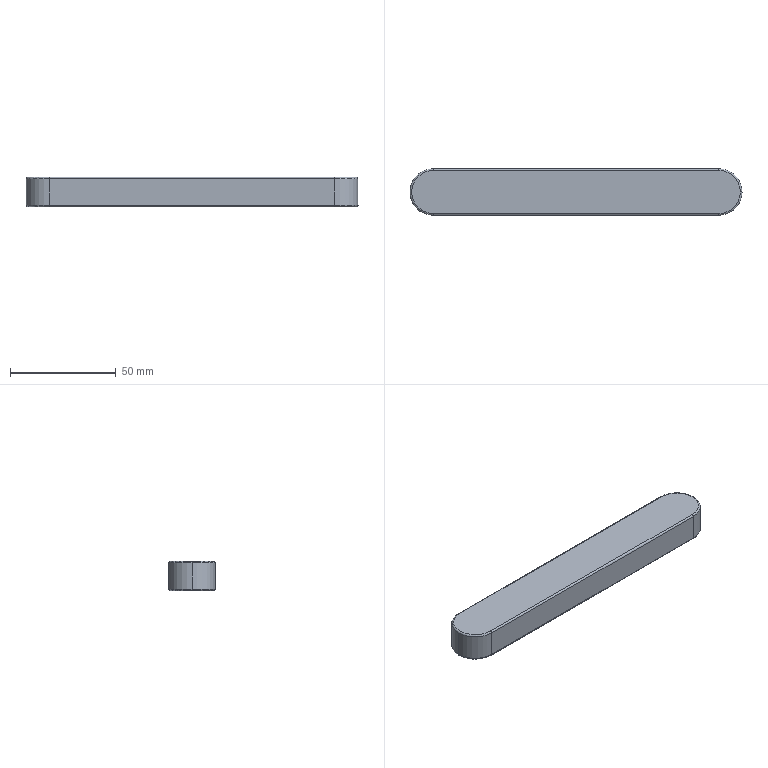Part | SolidWorks | features Extrusion 1, Fillet 1 | 1 solid | 17 faces | box 157 x 22 x 14 mm | volume 46809 mm3 | cylinder 7 | torus 6 | plane 4 | commonest cylinder face diameters 1.6 x4 22 x3
STEP:
#1=CARTESIAN_POINT('',(77.7,0.,0.));
#2=VERTEX_POINT('',#1);
#3=CARTESIAN_POINT('',(67.5,-10.2,0.));
#4=VERTEX_POINT('',#3);
#5=CARTESIAN_POINT('',(67.5,0.,0.));
#6=DIRECTION('',(0.,0.,-1.));
#7=DIRECTION('',(1.,0.,0.));
#8=AXIS2_PLACEMENT_3D('',#5,#6,#7);
#9=CIRCLE('',#8,10.2);
#10=EDGE_CURVE('',#2,#4,#9,.T.);
#11=ORIENTED_EDGE('',*,*,#10,.F.);
#12=CARTESIAN_POINT('',(78.5,0.,0.8));
#13=VERTEX_POINT('',#12);
#14=CARTESIAN_POINT('',(77.7,0.,0.8));
#15=DIRECTION('',(0.,-1.,0.));
#16=DIRECTION('',(1.,0.,0.));
#17=AXIS2_PLACEMENT_3D('',#14,#15,#16);
#18=CIRCLE('',#17,0.8);
#19=EDGE_CURVE('',#2,#13,#18,.T.);
#20=ORIENTED_EDGE('',*,*,#19,.T.);
#21=CARTESIAN_POINT('',(67.5,-11.,0.8));
#22=VERTEX_POINT('',#21);
#23=CARTESIAN_POINT('',(67.5,0.,0.8));
#24=DIRECTION('',(0.,0.,1.));
#25=DIRECTION('',(1.,0.,0.));
#26=AXIS2_PLACEMENT_3D('',#23,#24,#25);
#27=CIRCLE('',#26,11.);
#28=EDGE_CURVE('',#22,#13,#27,.T.);
#29=ORIENTED_EDGE('',*,*,#28,.F.);
#30=CARTESIAN_POINT('',(67.5,-10.2,0.8));
#31=DIRECTION('',(1.,0.,0.));
#32=DIRECTION('',(0.,0.,-1.));
#33=AXIS2_PLACEMENT_3D('',#30,#31,#32);
#34=CIRCLE('',#33,0.8);
#35=EDGE_CURVE('',#22,#4,#34,.T.);
#36=ORIENTED_EDGE('',*,*,#35,.T.);
#37=EDGE_LOOP('',(#11,#20,#29,#36));
#38=FACE_OUTER_BOUND('',#37,.T.);
#39=CARTESIAN_POINT('',(67.5,0.,0.8));
#40=DIRECTION('',(0.,0.,1.));
#41=DIRECTION('',(1.,0.,0.));
#42=AXIS2_PLACEMENT_3D('',#39,#40,#41);
#43=TOROIDAL_SURFACE('',#42,10.2,0.8);
#44=ADVANCED_FACE('',(#38),#43,.T.);
#45=CARTESIAN_POINT('',(78.5,0.,13.2));
#46=VERTEX_POINT('',#45);
#47=CARTESIAN_POINT('',(67.5,-11.,13.2));
#48=VERTEX_POINT('',#47);
#49=CARTESIAN_POINT('',(67.5,0.,13.2));
#50=DIRECTION('',(0.,0.,-1.));
#51=DIRECTION('',(1.,0.,0.));
#52=AXIS2_PLACEMENT_3D('',#49,#50,#51);
#53=CIRCLE('',#52,11.);
#54=EDGE_CURVE('',#46,#48,#53,.T.);
#55=ORIENTED_EDGE('',*,*,#54,.F.);
#56=CARTESIAN_POINT('',(77.7,0.,14.));
#57=VERTEX_POINT('',#56);
#58=CARTESIAN_POINT('',(77.7,0.,13.2));
#59=DIRECTION('',(0.,-1.,0.));
#60=DIRECTION('',(1.,0.,0.));
#61=AXIS2_PLACEMENT_3D('',#58,#59,#60);
#62=CIRCLE('',#61,0.8);
#63=EDGE_CURVE('',#46,#57,#62,.T.);
#64=ORIENTED_EDGE('',*,*,#63,.T.);
#65=CARTESIAN_POINT('',(67.5,-10.2,14.));
#66=VERTEX_POINT('',#65);
#67=CARTESIAN_POINT('',(67.5,0.,14.));
#68=DIRECTION('',(0.,0.,1.));
#69=DIRECTION('',(1.,0.,0.));
#70=AXIS2_PLACEMENT_3D('',#67,#68,#69);
#71=CIRCLE('',#70,10.2);
#72=EDGE_CURVE('',#66,#57,#71,.T.);
#73=ORIENTED_EDGE('',*,*,#72,.F.);
#74=CARTESIAN_POINT('',(67.5,-10.2,13.2));
#75=DIRECTION('',(1.,0.,0.));
#76=DIRECTION('',(0.,0.,-1.));
#77=AXIS2_PLACEMENT_3D('',#74,#75,#76);
#78=CIRCLE('',#77,0.8);
#79=EDGE_CURVE('',#66,#48,#78,.T.);
#80=ORIENTED_EDGE('',*,*,#79,.T.);
#81=EDGE_LOOP('',(#55,#64,#73,#80));
#82=FACE_OUTER_BOUND('',#81,.T.);
#83=CARTESIAN_POINT('',(67.5,0.,13.2));
#84=DIRECTION('',(0.,0.,1.));
#85=DIRECTION('',(1.,0.,0.));
#86=AXIS2_PLACEMENT_3D('',#83,#84,#85);
#87=TOROIDAL_SURFACE('',#86,10.2,0.8);
#88=ADVANCED_FACE('',(#82),#87,.T.);
#89=CARTESIAN_POINT('',(-67.5,-11.,13.2));
#90=VERTEX_POINT('',#89);
#91=CARTESIAN_POINT('',(-78.5,0.,13.2));
#92=VERTEX_POINT('',#91);
#93=CARTESIAN_POINT('',(-67.5,0.,13.2));
#94=DIRECTION('',(0.,0.,-1.));
#95=DIRECTION('',(1.,0.,0.));
#96=AXIS2_PLACEMENT_3D('',#93,#94,#95);
#97=CIRCLE('',#96,11.);
#98=EDGE_CURVE('',#90,#92,#97,.T.);
#99=ORIENTED_EDGE('',*,*,#98,.T.);
#100=CARTESIAN_POINT('',(-78.5,0.,0.8));
#101=VERTEX_POINT('',#100);
#102=CARTESIAN_POINT('',(-78.5,0.,14.));
#103=DIRECTION('',(0.,0.,-1.));
#104=VECTOR('',#103,1000.);
#105=LINE('',#102,#104);
#106=EDGE_CURVE('',#92,#101,#105,.T.);
#107=ORIENTED_EDGE('',*,*,#106,.T.);
#108=CARTESIAN_POINT('',(-67.5,-11.,0.8));
#109=VERTEX_POINT('',#108);
#110=CARTESIAN_POINT('',(-67.5,0.,0.8));
#111=DIRECTION('',(0.,0.,1.));
#112=DIRECTION('',(1.,0.,0.));
#113=AXIS2_PLACEMENT_3D('',#110,#111,#112);
#114=CIRCLE('',#113,11.);
#115=EDGE_CURVE('',#101,#109,#114,.T.);
#116=ORIENTED_EDGE('',*,*,#115,.T.);
#117=CARTESIAN_POINT('',(-67.5,-11.,14.));
#118=DIRECTION('',(0.,0.,-1.));
#119=VECTOR('',#118,1000.);
#120=LINE('',#117,#119);
#121=EDGE_CURVE('',#90,#109,#120,.T.);
#122=ORIENTED_EDGE('',*,*,#121,.F.);
#123=EDGE_LOOP('',(#99,#107,#116,#122));
#124=FACE_OUTER_BOUND('',#123,.T.);
#125=CARTESIAN_POINT('',(-67.5,0.,14.));
#126=DIRECTION('',(0.,0.,-1.));
#127=DIRECTION('',(-1.,0.,0.));
#128=AXIS2_PLACEMENT_3D('',#125,#126,#127);
#129=CYLINDRICAL_SURFACE('',#128,11.);
#130=ADVANCED_FACE('',(#124),#129,.T.);
#131=ORIENTED_EDGE('',*,*,#106,.F.);
#132=CARTESIAN_POINT('',(-67.5,11.,13.2));
#133=VERTEX_POINT('',#132);
#134=CARTESIAN_POINT('',(-67.5,0.,13.2));
#135=DIRECTION('',(0.,0.,-1.));
#136=DIRECTION('',(1.,0.,0.));
#137=AXIS2_PLACEMENT_3D('',#134,#135,#136);
#138=CIRCLE('',#137,11.);
#139=EDGE_CURVE('',#92,#133,#138,.T.);
#140=ORIENTED_EDGE('',*,*,#139,.T.);
#141=CARTESIAN_POINT('',(-67.5,11.,0.8));
#142=VERTEX_POINT('',#141);
#143=CARTESIAN_POINT('',(-67.5,11.,14.));
#144=DIRECTION('',(0.,0.,-1.));
#145=VECTOR('',#144,1000.);
#146=LINE('',#143,#145);
#147=EDGE_CURVE('',#133,#142,#146,.T.);
#148=ORIENTED_EDGE('',*,*,#147,.T.);
#149=CARTESIAN_POINT('',(-67.5,0.,0.8));
#150=DIRECTION('',(0.,0.,1.));
#151=DIRECTION('',(1.,0.,0.));
#152=AXIS2_PLACEMENT_3D('',#149,#150,#151);
#153=CIRCLE('',#152,11.);
#154=EDGE_CURVE('',#142,#101,#153,.T.);
#155=ORIENTED_EDGE('',*,*,#154,.T.);
#156=EDGE_LOOP('',(#131,#140,#148,#155));
#157=FACE_OUTER_BOUND('',#156,.T.);
#158=CARTESIAN_POINT('',(-67.5,0.,14.));
#159=DIRECTION('',(0.,0.,-1.));
#160=DIRECTION('',(-1.,0.,0.));
#161=AXIS2_PLACEMENT_3D('',#158,#159,#160);
#162=CYLINDRICAL_SURFACE('',#161,11.);
#163=ADVANCED_FACE('',(#157),#162,.T.);
#164=CARTESIAN_POINT('',(67.5,-11.,14.));
#165=DIRECTION('',(0.,0.,-1.));
#166=VECTOR('',#165,1000.);
#167=LINE('',#164,#166);
#168=EDGE_CURVE('',#48,#22,#167,.T.);
#169=ORIENTED_EDGE('',*,*,#168,.F.);
#170=CARTESIAN_POINT('',(-67.5,-11.,13.2));
#171=DIRECTION('',(-1.,0.,0.));
#172=VECTOR('',#171,1000.);
#173=LINE('',#170,#172);
#174=EDGE_CURVE('',#48,#90,#173,.T.);
#175=ORIENTED_EDGE('',*,*,#174,.T.);
#176=ORIENTED_EDGE('',*,*,#121,.T.);
#177=CARTESIAN_POINT('',(-67.5,-11.,0.8));
#178=DIRECTION('',(1.,0.,0.));
#179=VECTOR('',#178,1000.);
#180=LINE('',#177,#179);
#181=EDGE_CURVE('',#109,#22,#180,.T.);
#182=ORIENTED_EDGE('',*,*,#181,.T.);
#183=EDGE_LOOP('',(#169,#175,#176,#182));
#184=FACE_OUTER_BOUND('',#183,.T.);
#185=CARTESIAN_POINT('',(-67.5,-11.,14.));
#186=DIRECTION('',(0.,1.,0.));
#187=DIRECTION('',(-1.,0.,0.));
#188=AXIS2_PLACEMENT_3D('',#185,#186,#187);
#189=PLANE('',#188);
#190=ADVANCED_FACE('',(#184),#189,.F.);
#191=CARTESIAN_POINT('',(67.5,11.,13.2));
#192=VERTEX_POINT('',#191);
#193=CARTESIAN_POINT('',(67.5,11.,0.8));
#194=VERTEX_POINT('',#193);
#195=CARTESIAN_POINT('',(67.5,11.,14.));
#196=DIRECTION('',(0.,0.,-1.));
#197=VECTOR('',#196,1000.);
#198=LINE('',#195,#197);
#199=EDGE_CURVE('',#192,#194,#198,.T.);
#200=ORIENTED_EDGE('',*,*,#199,.F.);
#201=CARTESIAN_POINT('',(67.5,0.,13.2));
#202=DIRECTION('',(0.,0.,-1.));
#203=DIRECTION('',(1.,0.,0.));
#204=AXIS2_PLACEMENT_3D('',#201,#202,#203);
#205=CIRCLE('',#204,11.);
#206=EDGE_CURVE('',#192,#46,#205,.T.);
#207=ORIENTED_EDGE('',*,*,#206,.T.);
#208=ORIENTED_EDGE('',*,*,#54,.T.);
#209=ORIENTED_EDGE('',*,*,#168,.T.);
#210=ORIENTED_EDGE('',*,*,#28,.T.);
#211=CARTESIAN_POINT('',(67.5,0.,0.8));
#212=DIRECTION('',(0.,0.,1.));
#213=DIRECTION('',(1.,0.,0.));
#214=AXIS2_PLACEMENT_3D('',#211,#212,#213);
#215=CIRCLE('',#214,11.);
#216=EDGE_CURVE('',#13,#194,#215,.T.);
#217=ORIENTED_EDGE('',*,*,#216,.T.);
#218=EDGE_LOOP('',(#200,#207,#208,#209,#210,#217));
#219=FACE_OUTER_BOUND('',#218,.T.);
#220=CARTESIAN_POINT('',(67.5,0.,14.));
#221=DIRECTION('',(0.,0.,-1.));
#222=DIRECTION('',(-1.,0.,0.));
#223=AXIS2_PLACEMENT_3D('',#220,#221,#222);
#224=CYLINDRICAL_SURFACE('',#223,11.);
#225=ADVANCED_FACE('',(#219),#224,.T.);
#226=ORIENTED_EDGE('',*,*,#147,.F.);
#227=CARTESIAN_POINT('',(67.5,11.,13.2));
#228=DIRECTION('',(1.,0.,0.));
#229=VECTOR('',#228,1000.);
#230=LINE('',#227,#229);
#231=EDGE_CURVE('',#133,#192,#230,.T.);
#232=ORIENTED_EDGE('',*,*,#231,.T.);
#233=ORIENTED_EDGE('',*,*,#199,.T.);
#234=CARTESIAN_POINT('',(-67.5,11.,0.8));
#235=DIRECTION('',(-1.,0.,0.));
#236=VECTOR('',#235,1000.);
#237=LINE('',#234,#236);
#238=EDGE_CURVE('',#194,#142,#237,.T.);
#239=ORIENTED_EDGE('',*,*,#238,.T.);
#240=EDGE_LOOP('',(#226,#232,#233,#239));
#241=FACE_OUTER_BOUND('',#240,.T.);
#242=CARTESIAN_POINT('',(-67.5,11.,14.));
#243=DIRECTION('',(0.,-1.,0.));
#244=DIRECTION('',(1.,0.,0.));
#245=AXIS2_PLACEMENT_3D('',#242,#243,#244);
#246=PLANE('',#245);
#247=ADVANCED_FACE('',(#241),#246,.F.);
#248=CARTESIAN_POINT('',(-67.5,-10.2,14.));
#249=VERTEX_POINT('',#248);
#250=CARTESIAN_POINT('',(67.5,-10.2,14.));
#251=DIRECTION('',(1.,0.,0.));
#252=VECTOR('',#251,1000.);
#253=LINE('',#250,#252);
#254=EDGE_CURVE('',#249,#66,#253,.T.);
#255=ORIENTED_EDGE('',*,*,#254,.T.);
#256=ORIENTED_EDGE('',*,*,#72,.T.);
#257=CARTESIAN_POINT('',(67.5,10.2,14.));
#258=VERTEX_POINT('',#257);
#259=CARTESIAN_POINT('',(67.5,0.,14.));
#260=DIRECTION('',(0.,0.,1.));
#261=DIRECTION('',(1.,0.,0.));
#262=AXIS2_PLACEMENT_3D('',#259,#260,#261);
#263=CIRCLE('',#262,10.2);
#264=EDGE_CURVE('',#57,#258,#263,.T.);
#265=ORIENTED_EDGE('',*,*,#264,.T.);
#266=CARTESIAN_POINT('',(-67.5,10.2,14.));
#267=VERTEX_POINT('',#266);
#268=CARTESIAN_POINT('',(-67.5,10.2,14.));
#269=DIRECTION('',(-1.,0.,0.));
#270=VECTOR('',#269,1000.);
#271=LINE('',#268,#270);
#272=EDGE_CURVE('',#258,#267,#271,.T.);
#273=ORIENTED_EDGE('',*,*,#272,.T.);
#274=CARTESIAN_POINT('',(-67.5,0.,14.));
#275=DIRECTION('',(0.,0.,1.));
#276=DIRECTION('',(1.,0.,0.));
#277=AXIS2_PLACEMENT_3D('',#274,#275,#276);
#278=CIRCLE('',#277,10.2);
#279=EDGE_CURVE('',#267,#249,#278,.T.);
#280=ORIENTED_EDGE('',*,*,#279,.T.);
#281=EDGE_LOOP('',(#255,#256,#265,#273,#280));
#282=FACE_OUTER_BOUND('',#281,.T.);
#283=CARTESIAN_POINT('',(-67.5,0.,14.));
#284=DIRECTION('',(0.,0.,1.));
#285=DIRECTION('',(1.,0.,0.));
#286=AXIS2_PLACEMENT_3D('',#283,#284,#285);
#287=PLANE('',#286);
#288=ADVANCED_FACE('',(#282),#287,.T.);
#289=CARTESIAN_POINT('',(-67.5,10.2,0.));
#290=VERTEX_POINT('',#289);
#291=CARTESIAN_POINT('',(67.5,10.2,0.));
#292=VERTEX_POINT('',#291);
#293=CARTESIAN_POINT('',(-67.5,10.2,0.));
#294=DIRECTION('',(1.,0.,0.));
#295=VECTOR('',#294,1000.);
#296=LINE('',#293,#295);
#297=EDGE_CURVE('',#290,#292,#296,.T.);
#298=ORIENTED_EDGE('',*,*,#297,.T.);
#299=CARTESIAN_POINT('',(67.5,0.,0.));
#300=DIRECTION('',(0.,0.,-1.));
#301=DIRECTION('',(1.,0.,0.));
#302=AXIS2_PLACEMENT_3D('',#299,#300,#301);
#303=CIRCLE('',#302,10.2);
#304=EDGE_CURVE('',#292,#2,#303,.T.);
#305=ORIENTED_EDGE('',*,*,#304,.T.);
#306=ORIENTED_EDGE('',*,*,#10,.T.);
#307=CARTESIAN_POINT('',(-67.5,-10.2,0.));
#308=VERTEX_POINT('',#307);
#309=CARTESIAN_POINT('',(-67.5,-10.2,0.));
#310=DIRECTION('',(-1.,0.,0.));
#311=VECTOR('',#310,1000.);
#312=LINE('',#309,#311);
#313=EDGE_CURVE('',#4,#308,#312,.T.);
#314=ORIENTED_EDGE('',*,*,#313,.T.);
#315=CARTESIAN_POINT('',(-67.5,0.,0.));
#316=DIRECTION('',(0.,0.,-1.));
#317=DIRECTION('',(1.,0.,0.));
#318=AXIS2_PLACEMENT_3D('',#315,#316,#317);
#319=CIRCLE('',#318,10.2);
#320=EDGE_CURVE('',#308,#290,#319,.T.);
#321=ORIENTED_EDGE('',*,*,#320,.T.);
#322=EDGE_LOOP('',(#298,#305,#306,#314,#321));
#323=FACE_OUTER_BOUND('',#322,.T.);
#324=CARTESIAN_POINT('',(-67.5,0.,0.));
#325=DIRECTION('',(0.,0.,1.));
#326=DIRECTION('',(1.,0.,0.));
#327=AXIS2_PLACEMENT_3D('',#324,#325,#326);
#328=PLANE('',#327);
#329=ADVANCED_FACE('',(#323),#328,.F.);
#330=CARTESIAN_POINT('',(-67.5,10.2,13.2));
#331=DIRECTION('',(1.,0.,0.));
#332=DIRECTION('',(0.,0.,-1.));
#333=AXIS2_PLACEMENT_3D('',#330,#331,#332);
#334=CIRCLE('',#333,0.8);
#335=EDGE_CURVE('',#133,#267,#334,.T.);
#336=ORIENTED_EDGE('',*,*,#335,.F.);
#337=ORIENTED_EDGE('',*,*,#139,.F.);
#338=ORIENTED_EDGE('',*,*,#98,.F.);
#339=CARTESIAN_POINT('',(-67.5,-10.2,13.2));
#340=DIRECTION('',(1.,0.,0.));
#341=DIRECTION('',(0.,0.,-1.));
#342=AXIS2_PLACEMENT_3D('',#339,#340,#341);
#343=CIRCLE('',#342,0.8);
#344=EDGE_CURVE('',#249,#90,#343,.T.);
#345=ORIENTED_EDGE('',*,*,#344,.F.);
#346=ORIENTED_EDGE('',*,*,#279,.F.);
#347=EDGE_LOOP('',(#336,#337,#338,#345,#346));
#348=FACE_OUTER_BOUND('',#347,.T.);
#349=CARTESIAN_POINT('',(-67.5,0.,13.2));
#350=DIRECTION('',(0.,0.,1.));
#351=DIRECTION('',(1.,0.,0.));
#352=AXIS2_PLACEMENT_3D('',#349,#350,#351);
#353=TOROIDAL_SURFACE('',#352,10.2,0.8);
#354=ADVANCED_FACE('',(#348),#353,.T.);
#355=ORIENTED_EDGE('',*,*,#344,.T.);
#356=ORIENTED_EDGE('',*,*,#174,.F.);
#357=ORIENTED_EDGE('',*,*,#79,.F.);
#358=ORIENTED_EDGE('',*,*,#254,.F.);
#359=EDGE_LOOP('',(#355,#356,#357,#358));
#360=FACE_OUTER_BOUND('',#359,.T.);
#361=CARTESIAN_POINT('',(-67.5,-10.2,13.2));
#362=DIRECTION('',(-1.,0.,0.));
#363=DIRECTION('',(0.,-1.,0.));
#364=AXIS2_PLACEMENT_3D('',#361,#362,#363);
#365=CYLINDRICAL_SURFACE('',#364,0.8);
#366=ADVANCED_FACE('',(#360),#365,.T.);
#367=ORIENTED_EDGE('',*,*,#335,.T.);
#368=ORIENTED_EDGE('',*,*,#272,.F.);
#369=CARTESIAN_POINT('',(67.5,10.2,13.2));
#370=DIRECTION('',(1.,0.,0.));
#371=DIRECTION('',(0.,0.,-1.));
#372=AXIS2_PLACEMENT_3D('',#369,#370,#371);
#373=CIRCLE('',#372,0.8);
#374=EDGE_CURVE('',#192,#258,#373,.T.);
#375=ORIENTED_EDGE('',*,*,#374,.F.);
#376=ORIENTED_EDGE('',*,*,#231,.F.);
#377=EDGE_LOOP('',(#367,#368,#375,#376));
#378=FACE_OUTER_BOUND('',#377,.T.);
#379=CARTESIAN_POINT('',(-67.5,10.2,13.2));
#380=DIRECTION('',(1.,0.,0.));
#381=DIRECTION('',(0.,1.,0.));
#382=AXIS2_PLACEMENT_3D('',#379,#380,#381);
#383=CYLINDRICAL_SURFACE('',#382,0.8);
#384=ADVANCED_FACE('',(#378),#383,.T.);
#385=ORIENTED_EDGE('',*,*,#63,.F.);
#386=ORIENTED_EDGE('',*,*,#206,.F.);
#387=ORIENTED_EDGE('',*,*,#374,.T.);
#388=ORIENTED_EDGE('',*,*,#264,.F.);
#389=EDGE_LOOP('',(#385,#386,#387,#388));
#390=FACE_OUTER_BOUND('',#389,.T.);
#391=CARTESIAN_POINT('',(67.5,0.,13.2));
#392=DIRECTION('',(0.,0.,1.));
#393=DIRECTION('',(1.,0.,0.));
#394=AXIS2_PLACEMENT_3D('',#391,#392,#393);
#395=TOROIDAL_SURFACE('',#394,10.2,0.8);
#396=ADVANCED_FACE('',(#390),#395,.T.);
#397=CARTESIAN_POINT('',(-67.5,10.2,0.8));
#398=DIRECTION('',(1.,0.,0.));
#399=DIRECTION('',(0.,0.,-1.));
#400=AXIS2_PLACEMENT_3D('',#397,#398,#399);
#401=CIRCLE('',#400,0.8);
#402=EDGE_CURVE('',#290,#142,#401,.T.);
#403=ORIENTED_EDGE('',*,*,#402,.F.);
#404=ORIENTED_EDGE('',*,*,#320,.F.);
#405=CARTESIAN_POINT('',(-67.5,-10.2,0.8));
#406=DIRECTION('',(1.,0.,0.));
#407=DIRECTION('',(0.,0.,-1.));
#408=AXIS2_PLACEMENT_3D('',#405,#406,#407);
#409=CIRCLE('',#408,0.8);
#410=EDGE_CURVE('',#109,#308,#409,.T.);
#411=ORIENTED_EDGE('',*,*,#410,.F.);
#412=ORIENTED_EDGE('',*,*,#115,.F.);
#413=ORIENTED_EDGE('',*,*,#154,.F.);
#414=EDGE_LOOP('',(#403,#404,#411,#412,#413));
#415=FACE_OUTER_BOUND('',#414,.T.);
#416=CARTESIAN_POINT('',(-67.5,0.,0.8));
#417=DIRECTION('',(0.,0.,1.));
#418=DIRECTION('',(1.,0.,0.));
#419=AXIS2_PLACEMENT_3D('',#416,#417,#418);
#420=TOROIDAL_SURFACE('',#419,10.2,0.8);
#421=ADVANCED_FACE('',(#415),#420,.T.);
#422=ORIENTED_EDGE('',*,*,#410,.T.);
#423=ORIENTED_EDGE('',*,*,#313,.F.);
#424=ORIENTED_EDGE('',*,*,#35,.F.);
#425=ORIENTED_EDGE('',*,*,#181,.F.);
#426=EDGE_LOOP('',(#422,#423,#424,#425));
#427=FACE_OUTER_BOUND('',#426,.T.);
#428=CARTESIAN_POINT('',(-67.5,-10.2,0.8));
#429=DIRECTION('',(1.,0.,0.));
#430=DIRECTION('',(0.,1.,0.));
#431=AXIS2_PLACEMENT_3D('',#428,#429,#430);
#432=CYLINDRICAL_SURFACE('',#431,0.8);
#433=ADVANCED_FACE('',(#427),#432,.T.);
#434=ORIENTED_EDGE('',*,*,#402,.T.);
#435=ORIENTED_EDGE('',*,*,#238,.F.);
#436=CARTESIAN_POINT('',(67.5,10.2,0.8));
#437=DIRECTION('',(1.,0.,0.));
#438=DIRECTION('',(0.,0.,-1.));
#439=AXIS2_PLACEMENT_3D('',#436,#437,#438);
#440=CIRCLE('',#439,0.8);
#441=EDGE_CURVE('',#292,#194,#440,.T.);
#442=ORIENTED_EDGE('',*,*,#441,.F.);
#443=ORIENTED_EDGE('',*,*,#297,.F.);
#444=EDGE_LOOP('',(#434,#435,#442,#443));
#445=FACE_OUTER_BOUND('',#444,.T.);
#446=CARTESIAN_POINT('',(-67.5,10.2,0.8));
#447=DIRECTION('',(-1.,0.,0.));
#448=DIRECTION('',(0.,-1.,0.));
#449=AXIS2_PLACEMENT_3D('',#446,#447,#448);
#450=CYLINDRICAL_SURFACE('',#449,0.8);
#451=ADVANCED_FACE('',(#445),#450,.T.);
#452=ORIENTED_EDGE('',*,*,#19,.F.);
#453=ORIENTED_EDGE('',*,*,#304,.F.);
#454=ORIENTED_EDGE('',*,*,#441,.T.);
#455=ORIENTED_EDGE('',*,*,#216,.F.);
#456=EDGE_LOOP('',(#452,#453,#454,#455));
#457=FACE_OUTER_BOUND('',#456,.T.);
#458=CARTESIAN_POINT('',(67.5,0.,0.8));
#459=DIRECTION('',(0.,0.,1.));
#460=DIRECTION('',(1.,0.,0.));
#461=AXIS2_PLACEMENT_3D('',#458,#459,#460);
#462=TOROIDAL_SURFACE('',#461,10.2,0.8);
#463=ADVANCED_FACE('',(#457),#462,.T.);
#464=CLOSED_SHELL('',(#44,#88,#130,#163,#190,#225,#247,#288,#329,#354,#366,#384,#396,#421,#433,#451,#463));
#465=MANIFOLD_SOLID_BREP('',#464);
#466=CARTESIAN_POINT('',(0.,0.,0.));
#467=DIRECTION('',(0.,0.,1.));
#468=DIRECTION('',(1.,0.,0.));
#469=AXIS2_PLACEMENT_3D('',#466,#467,#468);
#470=(LENGTH_UNIT()NAMED_UNIT(*)SI_UNIT(.MILLI.,.METRE.));
#471=UNCERTAINTY_MEASURE_WITH_UNIT(LENGTH_MEASURE(0.00001),#470,'','');
#472=(NAMED_UNIT(*)PLANE_ANGLE_UNIT()SI_UNIT($,.RADIAN.));
#473=(NAMED_UNIT(*)SI_UNIT($,.STERADIAN.)SOLID_ANGLE_UNIT());
#474=(GEOMETRIC_REPRESENTATION_CONTEXT(3)GLOBAL_UNCERTAINTY_ASSIGNED_CONTEXT((#471))GLOBAL_UNIT_ASSIGNED_CONTEXT((#470,#472,#473))REPRESENTATION_CONTEXT('',''));
#475=ADVANCED_BREP_SHAPE_REPRESENTATION('',(#465,#469),#474);